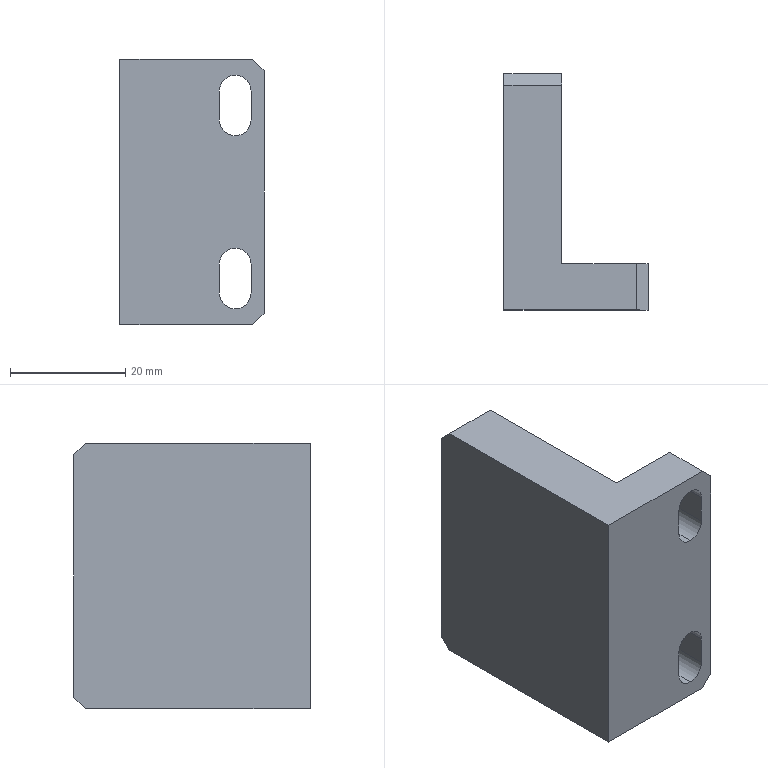Part | SolidWorks | features Chamfer 1, Extrusion 1, HoleWzd 1, ICE 1 | 1 solid | 30 faces | box 25 x 41 x 46 mm | volume 23309 mm3 | plane 16 | cylinder 10 | cone 4 | commonest cylinder face diameters 5.5 x6 3.3 x4
STEP:
#1=CARTESIAN_POINT('',(5.,30.9,-19.15));
#2=VERTEX_POINT('',#1);
#3=CARTESIAN_POINT('',(5.,30.9,-15.85));
#4=VERTEX_POINT('',#3);
#5=CARTESIAN_POINT('',(5.,30.9,-17.5));
#6=DIRECTION('',(0.,1.,0.));
#7=DIRECTION('',(0.,0.,1.));
#8=AXIS2_PLACEMENT_3D('',#5,#6,#7);
#9=CIRCLE('',#8,1.65);
#10=EDGE_CURVE('',#2,#4,#9,.T.);
#11=ORIENTED_EDGE('',*,*,#10,.F.);
#12=CARTESIAN_POINT('',(5.,41.,-19.15));
#13=VERTEX_POINT('',#12);
#14=CARTESIAN_POINT('',(5.,41.,-19.15));
#15=DIRECTION('',(0.,1.,0.));
#16=VECTOR('',#15,1000.);
#17=LINE('',#14,#16);
#18=EDGE_CURVE('',#2,#13,#17,.T.);
#19=ORIENTED_EDGE('',*,*,#18,.T.);
#20=CARTESIAN_POINT('',(5.,41.,-15.85));
#21=VERTEX_POINT('',#20);
#22=CARTESIAN_POINT('',(5.,41.,-17.5));
#23=DIRECTION('',(0.,1.,0.));
#24=DIRECTION('',(0.,0.,1.));
#25=AXIS2_PLACEMENT_3D('',#22,#23,#24);
#26=CIRCLE('',#25,1.65);
#27=EDGE_CURVE('',#13,#21,#26,.T.);
#28=ORIENTED_EDGE('',*,*,#27,.T.);
#29=CARTESIAN_POINT('',(5.,41.,-15.85));
#30=DIRECTION('',(0.,1.,0.));
#31=VECTOR('',#30,1000.);
#32=LINE('',#29,#31);
#33=EDGE_CURVE('',#4,#21,#32,.T.);
#34=ORIENTED_EDGE('',*,*,#33,.F.);
#35=EDGE_LOOP('',(#11,#19,#28,#34));
#36=FACE_OUTER_BOUND('',#35,.T.);
#37=CARTESIAN_POINT('',(5.,41.,-17.5));
#38=DIRECTION('',(0.,1.,0.));
#39=DIRECTION('',(0.,0.,1.));
#40=AXIS2_PLACEMENT_3D('',#37,#38,#39);
#41=CYLINDRICAL_SURFACE('',#40,1.65);
#42=ADVANCED_FACE('',(#36),#41,.F.);
#43=CARTESIAN_POINT('',(5.,29.909,-17.5));
#44=VERTEX_POINT('',#43);
#45=CARTESIAN_POINT('',(5.,30.9,-15.85));
#46=DIRECTION('',(0.,0.515,0.8572));
#47=VECTOR('',#46,1000.);
#48=LINE('',#45,#47);
#49=EDGE_CURVE('',#44,#4,#48,.T.);
#50=ORIENTED_EDGE('',*,*,#49,.F.);
#51=CARTESIAN_POINT('',(5.,30.9,-19.15));
#52=DIRECTION('',(0.,0.515,-0.8572));
#53=VECTOR('',#52,1000.);
#54=LINE('',#51,#53);
#55=EDGE_CURVE('',#44,#2,#54,.T.);
#56=ORIENTED_EDGE('',*,*,#55,.T.);
#57=ORIENTED_EDGE('',*,*,#10,.T.);
#58=EDGE_LOOP('',(#50,#56,#57));
#59=FACE_OUTER_BOUND('',#58,.T.);
#60=CARTESIAN_POINT('',(5.,30.9,-17.5));
#61=DIRECTION('',(0.,1.,0.));
#62=DIRECTION('',(0.,0.,1.));
#63=AXIS2_PLACEMENT_3D('',#60,#61,#62);
#64=CONICAL_SURFACE('',#63,1.65,1.03);
#65=ADVANCED_FACE('',(#59),#64,.F.);
#66=CARTESIAN_POINT('',(5.,30.9,15.85));
#67=VERTEX_POINT('',#66);
#68=CARTESIAN_POINT('',(5.,30.9,19.15));
#69=VERTEX_POINT('',#68);
#70=CARTESIAN_POINT('',(5.,30.9,17.5));
#71=DIRECTION('',(0.,1.,0.));
#72=DIRECTION('',(0.,0.,1.));
#73=AXIS2_PLACEMENT_3D('',#70,#71,#72);
#74=CIRCLE('',#73,1.65);
#75=EDGE_CURVE('',#67,#69,#74,.T.);
#76=ORIENTED_EDGE('',*,*,#75,.F.);
#77=CARTESIAN_POINT('',(5.,41.,15.85));
#78=VERTEX_POINT('',#77);
#79=CARTESIAN_POINT('',(5.,41.,15.85));
#80=DIRECTION('',(0.,1.,0.));
#81=VECTOR('',#80,1000.);
#82=LINE('',#79,#81);
#83=EDGE_CURVE('',#67,#78,#82,.T.);
#84=ORIENTED_EDGE('',*,*,#83,.T.);
#85=CARTESIAN_POINT('',(5.,41.,19.15));
#86=VERTEX_POINT('',#85);
#87=CARTESIAN_POINT('',(5.,41.,17.5));
#88=DIRECTION('',(0.,1.,0.));
#89=DIRECTION('',(0.,0.,1.));
#90=AXIS2_PLACEMENT_3D('',#87,#88,#89);
#91=CIRCLE('',#90,1.65);
#92=EDGE_CURVE('',#78,#86,#91,.T.);
#93=ORIENTED_EDGE('',*,*,#92,.T.);
#94=CARTESIAN_POINT('',(5.,41.,19.15));
#95=DIRECTION('',(0.,1.,0.));
#96=VECTOR('',#95,1000.);
#97=LINE('',#94,#96);
#98=EDGE_CURVE('',#69,#86,#97,.T.);
#99=ORIENTED_EDGE('',*,*,#98,.F.);
#100=EDGE_LOOP('',(#76,#84,#93,#99));
#101=FACE_OUTER_BOUND('',#100,.T.);
#102=CARTESIAN_POINT('',(5.,41.,17.5));
#103=DIRECTION('',(0.,1.,0.));
#104=DIRECTION('',(0.,0.,1.));
#105=AXIS2_PLACEMENT_3D('',#102,#103,#104);
#106=CYLINDRICAL_SURFACE('',#105,1.65);
#107=ADVANCED_FACE('',(#101),#106,.F.);
#108=CARTESIAN_POINT('',(5.,29.909,17.5));
#109=VERTEX_POINT('',#108);
#110=CARTESIAN_POINT('',(5.,30.9,19.15));
#111=DIRECTION('',(0.,0.515,0.8572));
#112=VECTOR('',#111,1000.);
#113=LINE('',#110,#112);
#114=EDGE_CURVE('',#109,#69,#113,.T.);
#115=ORIENTED_EDGE('',*,*,#114,.F.);
#116=CARTESIAN_POINT('',(5.,30.9,15.85));
#117=DIRECTION('',(0.,0.515,-0.8572));
#118=VECTOR('',#117,1000.);
#119=LINE('',#116,#118);
#120=EDGE_CURVE('',#109,#67,#119,.T.);
#121=ORIENTED_EDGE('',*,*,#120,.T.);
#122=ORIENTED_EDGE('',*,*,#75,.T.);
#123=EDGE_LOOP('',(#115,#121,#122));
#124=FACE_OUTER_BOUND('',#123,.T.);
#125=CARTESIAN_POINT('',(5.,30.9,17.5));
#126=DIRECTION('',(0.,1.,0.));
#127=DIRECTION('',(0.,0.,1.));
#128=AXIS2_PLACEMENT_3D('',#125,#126,#127);
#129=CONICAL_SURFACE('',#128,1.65,1.03);
#130=ADVANCED_FACE('',(#124),#129,.F.);
#131=CARTESIAN_POINT('',(22.75,8.,12.5));
#132=VERTEX_POINT('',#131);
#133=CARTESIAN_POINT('',(20.,8.,9.75));
#134=VERTEX_POINT('',#133);
#135=CARTESIAN_POINT('',(20.,8.,12.5));
#136=DIRECTION('',(0.,1.,0.));
#137=DIRECTION('',(1.,0.,0.));
#138=AXIS2_PLACEMENT_3D('',#135,#136,#137);
#139=CIRCLE('',#138,2.75);
#140=EDGE_CURVE('',#132,#134,#139,.T.);
#141=ORIENTED_EDGE('',*,*,#140,.T.);
#142=CARTESIAN_POINT('',(20.,0.,9.75));
#143=VERTEX_POINT('',#142);
#144=CARTESIAN_POINT('',(20.,41.,9.75));
#145=DIRECTION('',(0.,-1.,0.));
#146=VECTOR('',#145,1000.);
#147=LINE('',#144,#146);
#148=EDGE_CURVE('',#134,#143,#147,.T.);
#149=ORIENTED_EDGE('',*,*,#148,.T.);
#150=CARTESIAN_POINT('',(22.75,0.,12.5));
#151=VERTEX_POINT('',#150);
#152=CARTESIAN_POINT('',(20.,0.,12.5));
#153=DIRECTION('',(0.,1.,0.));
#154=DIRECTION('',(0.,0.,1.));
#155=AXIS2_PLACEMENT_3D('',#152,#153,#154);
#156=CIRCLE('',#155,2.75);
#157=EDGE_CURVE('',#151,#143,#156,.T.);
#158=ORIENTED_EDGE('',*,*,#157,.F.);
#159=CARTESIAN_POINT('',(22.75,41.,12.5));
#160=DIRECTION('',(0.,-1.,0.));
#161=VECTOR('',#160,1000.);
#162=LINE('',#159,#161);
#163=EDGE_CURVE('',#132,#151,#162,.T.);
#164=ORIENTED_EDGE('',*,*,#163,.F.);
#165=EDGE_LOOP('',(#141,#149,#158,#164));
#166=FACE_OUTER_BOUND('',#165,.T.);
#167=CARTESIAN_POINT('',(20.,41.,12.5));
#168=DIRECTION('',(0.,-1.,0.));
#169=DIRECTION('',(0.,0.,-1.));
#170=AXIS2_PLACEMENT_3D('',#167,#168,#169);
#171=CYLINDRICAL_SURFACE('',#170,2.75);
#172=ADVANCED_FACE('',(#166),#171,.F.);
#173=CARTESIAN_POINT('',(22.75,8.,-17.5));
#174=VERTEX_POINT('',#173);
#175=CARTESIAN_POINT('',(20.,8.,-20.25));
#176=VERTEX_POINT('',#175);
#177=CARTESIAN_POINT('',(20.,8.,-17.5));
#178=DIRECTION('',(0.,1.,0.));
#179=DIRECTION('',(1.,0.,0.));
#180=AXIS2_PLACEMENT_3D('',#177,#178,#179);
#181=CIRCLE('',#180,2.75);
#182=EDGE_CURVE('',#174,#176,#181,.T.);
#183=ORIENTED_EDGE('',*,*,#182,.T.);
#184=CARTESIAN_POINT('',(20.,0.,-20.25));
#185=VERTEX_POINT('',#184);
#186=CARTESIAN_POINT('',(20.,41.,-20.25));
#187=DIRECTION('',(0.,-1.,0.));
#188=VECTOR('',#187,1000.);
#189=LINE('',#186,#188);
#190=EDGE_CURVE('',#176,#185,#189,.T.);
#191=ORIENTED_EDGE('',*,*,#190,.T.);
#192=CARTESIAN_POINT('',(22.75,0.,-17.5));
#193=VERTEX_POINT('',#192);
#194=CARTESIAN_POINT('',(20.,0.,-17.5));
#195=DIRECTION('',(0.,1.,0.));
#196=DIRECTION('',(0.,0.,1.));
#197=AXIS2_PLACEMENT_3D('',#194,#195,#196);
#198=CIRCLE('',#197,2.75);
#199=EDGE_CURVE('',#193,#185,#198,.T.);
#200=ORIENTED_EDGE('',*,*,#199,.F.);
#201=CARTESIAN_POINT('',(22.75,41.,-17.5));
#202=DIRECTION('',(0.,-1.,0.));
#203=VECTOR('',#202,1000.);
#204=LINE('',#201,#203);
#205=EDGE_CURVE('',#174,#193,#204,.T.);
#206=ORIENTED_EDGE('',*,*,#205,.F.);
#207=EDGE_LOOP('',(#183,#191,#200,#206));
#208=FACE_OUTER_BOUND('',#207,.T.);
#209=CARTESIAN_POINT('',(20.,41.,-17.5));
#210=DIRECTION('',(0.,-1.,0.));
#211=DIRECTION('',(0.,0.,-1.));
#212=AXIS2_PLACEMENT_3D('',#209,#210,#211);
#213=CYLINDRICAL_SURFACE('',#212,2.75);
#214=ADVANCED_FACE('',(#208),#213,.F.);
#215=ORIENTED_EDGE('',*,*,#199,.T.);
#216=CARTESIAN_POINT('',(17.25,0.,-17.5));
#217=VERTEX_POINT('',#216);
#218=CARTESIAN_POINT('',(20.,0.,-17.5));
#219=DIRECTION('',(0.,1.,0.));
#220=DIRECTION('',(0.,0.,1.));
#221=AXIS2_PLACEMENT_3D('',#218,#219,#220);
#222=CIRCLE('',#221,2.75);
#223=EDGE_CURVE('',#185,#217,#222,.T.);
#224=ORIENTED_EDGE('',*,*,#223,.T.);
#225=CARTESIAN_POINT('',(17.25,0.,-12.5));
#226=VERTEX_POINT('',#225);
#227=CARTESIAN_POINT('',(17.25,0.,-17.5));
#228=DIRECTION('',(0.,0.,1.));
#229=VECTOR('',#228,1000.);
#230=LINE('',#227,#229);
#231=EDGE_CURVE('',#217,#226,#230,.T.);
#232=ORIENTED_EDGE('',*,*,#231,.T.);
#233=CARTESIAN_POINT('',(22.75,0.,-12.5));
#234=VERTEX_POINT('',#233);
#235=CARTESIAN_POINT('',(20.,0.,-12.5));
#236=DIRECTION('',(0.,1.,0.));
#237=DIRECTION('',(0.,0.,1.));
#238=AXIS2_PLACEMENT_3D('',#235,#236,#237);
#239=CIRCLE('',#238,2.75);
#240=EDGE_CURVE('',#226,#234,#239,.T.);
#241=ORIENTED_EDGE('',*,*,#240,.T.);
#242=CARTESIAN_POINT('',(22.75,0.,-17.5));
#243=DIRECTION('',(0.,0.,-1.));
#244=VECTOR('',#243,1000.);
#245=LINE('',#242,#244);
#246=EDGE_CURVE('',#234,#193,#245,.T.);
#247=ORIENTED_EDGE('',*,*,#246,.T.);
#248=EDGE_LOOP('',(#215,#224,#232,#241,#247));
#249=FACE_BOUND('',#248,.T.);
#250=CARTESIAN_POINT('',(25.,0.,21.));
#251=VERTEX_POINT('',#250);
#252=CARTESIAN_POINT('',(25.,0.,-21.));
#253=VERTEX_POINT('',#252);
#254=CARTESIAN_POINT('',(25.,0.,23.));
#255=DIRECTION('',(0.,0.,-1.));
#256=VECTOR('',#255,1000.);
#257=LINE('',#254,#256);
#258=EDGE_CURVE('',#251,#253,#257,.T.);
#259=ORIENTED_EDGE('',*,*,#258,.F.);
#260=CARTESIAN_POINT('',(23.,0.,23.));
#261=VERTEX_POINT('',#260);
#262=CARTESIAN_POINT('',(23.,0.,23.));
#263=DIRECTION('',(-0.7071,0.,0.7071));
#264=VECTOR('',#263,1000.);
#265=LINE('',#262,#264);
#266=EDGE_CURVE('',#251,#261,#265,.T.);
#267=ORIENTED_EDGE('',*,*,#266,.T.);
#268=CARTESIAN_POINT('',(0.,0.,23.));
#269=VERTEX_POINT('',#268);
#270=CARTESIAN_POINT('',(0.,0.,23.));
#271=DIRECTION('',(1.,0.,0.));
#272=VECTOR('',#271,1000.);
#273=LINE('',#270,#272);
#274=EDGE_CURVE('',#269,#261,#273,.T.);
#275=ORIENTED_EDGE('',*,*,#274,.F.);
#276=CARTESIAN_POINT('',(0.,0.,-23.));
#277=VERTEX_POINT('',#276);
#278=CARTESIAN_POINT('',(0.,0.,23.));
#279=DIRECTION('',(0.,0.,-1.));
#280=VECTOR('',#279,1000.);
#281=LINE('',#278,#280);
#282=EDGE_CURVE('',#269,#277,#281,.T.);
#283=ORIENTED_EDGE('',*,*,#282,.T.);
#284=CARTESIAN_POINT('',(23.,0.,-23.));
#285=VERTEX_POINT('',#284);
#286=CARTESIAN_POINT('',(0.,0.,-23.));
#287=DIRECTION('',(1.,0.,0.));
#288=VECTOR('',#287,1000.);
#289=LINE('',#286,#288);
#290=EDGE_CURVE('',#277,#285,#289,.T.);
#291=ORIENTED_EDGE('',*,*,#290,.T.);
#292=CARTESIAN_POINT('',(25.,0.,-21.));
#293=DIRECTION('',(0.7071,0.,0.7071));
#294=VECTOR('',#293,1000.);
#295=LINE('',#292,#294);
#296=EDGE_CURVE('',#285,#253,#295,.T.);
#297=ORIENTED_EDGE('',*,*,#296,.T.);
#298=EDGE_LOOP('',(#259,#267,#275,#283,#291,#297));
#299=FACE_OUTER_BOUND('',#298,.T.);
#300=ORIENTED_EDGE('',*,*,#157,.T.);
#301=CARTESIAN_POINT('',(17.25,0.,12.5));
#302=VERTEX_POINT('',#301);
#303=CARTESIAN_POINT('',(20.,0.,12.5));
#304=DIRECTION('',(0.,1.,0.));
#305=DIRECTION('',(0.,0.,1.));
#306=AXIS2_PLACEMENT_3D('',#303,#304,#305);
#307=CIRCLE('',#306,2.75);
#308=EDGE_CURVE('',#143,#302,#307,.T.);
#309=ORIENTED_EDGE('',*,*,#308,.T.);
#310=CARTESIAN_POINT('',(17.25,0.,17.5));
#311=VERTEX_POINT('',#310);
#312=CARTESIAN_POINT('',(17.25,0.,12.5));
#313=DIRECTION('',(0.,0.,1.));
#314=VECTOR('',#313,1000.);
#315=LINE('',#312,#314);
#316=EDGE_CURVE('',#302,#311,#315,.T.);
#317=ORIENTED_EDGE('',*,*,#316,.T.);
#318=CARTESIAN_POINT('',(22.75,0.,17.5));
#319=VERTEX_POINT('',#318);
#320=CARTESIAN_POINT('',(20.,0.,17.5));
#321=DIRECTION('',(0.,1.,0.));
#322=DIRECTION('',(0.,0.,1.));
#323=AXIS2_PLACEMENT_3D('',#320,#321,#322);
#324=CIRCLE('',#323,2.75);
#325=EDGE_CURVE('',#311,#319,#324,.T.);
#326=ORIENTED_EDGE('',*,*,#325,.T.);
#327=CARTESIAN_POINT('',(22.75,0.,12.5));
#328=DIRECTION('',(0.,0.,-1.));
#329=VECTOR('',#328,1000.);
#330=LINE('',#327,#329);
#331=EDGE_CURVE('',#319,#151,#330,.T.);
#332=ORIENTED_EDGE('',*,*,#331,.T.);
#333=EDGE_LOOP('',(#300,#309,#317,#326,#332));
#334=FACE_BOUND('',#333,.T.);
#335=CARTESIAN_POINT('',(0.,0.,23.));
#336=DIRECTION('',(0.,1.,0.));
#337=DIRECTION('',(0.,0.,1.));
#338=AXIS2_PLACEMENT_3D('',#335,#336,#337);
#339=PLANE('',#338);
#340=ADVANCED_FACE('',(#249,#299,#334),#339,.F.);
#341=ORIENTED_EDGE('',*,*,#182,.F.);
#342=CARTESIAN_POINT('',(22.75,8.,-12.5));
#343=VERTEX_POINT('',#342);
#344=CARTESIAN_POINT('',(22.75,8.,23.));
#345=DIRECTION('',(0.,0.,-1.));
#346=VECTOR('',#345,1000.);
#347=LINE('',#344,#346);
#348=EDGE_CURVE('',#343,#174,#347,.T.);
#349=ORIENTED_EDGE('',*,*,#348,.F.);
#350=CARTESIAN_POINT('',(17.25,8.,-12.5));
#351=VERTEX_POINT('',#350);
#352=CARTESIAN_POINT('',(20.,8.,-12.5));
#353=DIRECTION('',(0.,1.,0.));
#354=DIRECTION('',(1.,0.,0.));
#355=AXIS2_PLACEMENT_3D('',#352,#353,#354);
#356=CIRCLE('',#355,2.75);
#357=EDGE_CURVE('',#351,#343,#356,.T.);
#358=ORIENTED_EDGE('',*,*,#357,.F.);
#359=CARTESIAN_POINT('',(17.25,8.,-17.5));
#360=VERTEX_POINT('',#359);
#361=CARTESIAN_POINT('',(17.25,8.,23.));
#362=DIRECTION('',(0.,0.,1.));
#363=VECTOR('',#362,1000.);
#364=LINE('',#361,#363);
#365=EDGE_CURVE('',#360,#351,#364,.T.);
#366=ORIENTED_EDGE('',*,*,#365,.F.);
#367=CARTESIAN_POINT('',(20.,8.,-17.5));
#368=DIRECTION('',(0.,1.,0.));
#369=DIRECTION('',(1.,0.,0.));
#370=AXIS2_PLACEMENT_3D('',#367,#368,#369);
#371=CIRCLE('',#370,2.75);
#372=EDGE_CURVE('',#176,#360,#371,.T.);
#373=ORIENTED_EDGE('',*,*,#372,.F.);
#374=EDGE_LOOP('',(#341,#349,#358,#366,#373));
#375=FACE_BOUND('',#374,.T.);
#376=CARTESIAN_POINT('',(23.,8.,23.));
#377=VERTEX_POINT('',#376);
#378=CARTESIAN_POINT('',(10.,8.,23.));
#379=VERTEX_POINT('',#378);
#380=CARTESIAN_POINT('',(25.,8.,23.));
#381=DIRECTION('',(-1.,0.,0.));
#382=VECTOR('',#381,1000.);
#383=LINE('',#380,#382);
#384=EDGE_CURVE('',#377,#379,#383,.T.);
#385=ORIENTED_EDGE('',*,*,#384,.F.);
#386=CARTESIAN_POINT('',(25.,8.,21.));
#387=VERTEX_POINT('',#386);
#388=CARTESIAN_POINT('',(23.,8.,23.));
#389=DIRECTION('',(0.7071,0.,-0.7071));
#390=VECTOR('',#389,1000.);
#391=LINE('',#388,#390);
#392=EDGE_CURVE('',#377,#387,#391,.T.);
#393=ORIENTED_EDGE('',*,*,#392,.T.);
#394=CARTESIAN_POINT('',(25.,8.,-21.));
#395=VERTEX_POINT('',#394);
#396=CARTESIAN_POINT('',(25.,8.,23.));
#397=DIRECTION('',(0.,0.,-1.));
#398=VECTOR('',#397,1000.);
#399=LINE('',#396,#398);
#400=EDGE_CURVE('',#387,#395,#399,.T.);
#401=ORIENTED_EDGE('',*,*,#400,.T.);
#402=CARTESIAN_POINT('',(23.,8.,-23.));
#403=VERTEX_POINT('',#402);
#404=CARTESIAN_POINT('',(25.,8.,-21.));
#405=DIRECTION('',(-0.7071,0.,-0.7071));
#406=VECTOR('',#405,1000.);
#407=LINE('',#404,#406);
#408=EDGE_CURVE('',#395,#403,#407,.T.);
#409=ORIENTED_EDGE('',*,*,#408,.T.);
#410=CARTESIAN_POINT('',(10.,8.,-23.));
#411=VERTEX_POINT('',#410);
#412=CARTESIAN_POINT('',(25.,8.,-23.));
#413=DIRECTION('',(-1.,0.,0.));
#414=VECTOR('',#413,1000.);
#415=LINE('',#412,#414);
#416=EDGE_CURVE('',#403,#411,#415,.T.);
#417=ORIENTED_EDGE('',*,*,#416,.T.);
#418=CARTESIAN_POINT('',(10.,8.,23.));
#419=DIRECTION('',(0.,0.,-1.));
#420=VECTOR('',#419,1000.);
#421=LINE('',#418,#420);
#422=EDGE_CURVE('',#379,#411,#421,.T.);
#423=ORIENTED_EDGE('',*,*,#422,.F.);
#424=EDGE_LOOP('',(#385,#393,#401,#409,#417,#423));
#425=FACE_OUTER_BOUND('',#424,.T.);
#426=ORIENTED_EDGE('',*,*,#140,.F.);
#427=CARTESIAN_POINT('',(22.75,8.,17.5));
#428=VERTEX_POINT('',#427);
#429=CARTESIAN_POINT('',(22.75,8.,23.));
#430=DIRECTION('',(0.,0.,-1.));
#431=VECTOR('',#430,1000.);
#432=LINE('',#429,#431);
#433=EDGE_CURVE('',#428,#132,#432,.T.);
#434=ORIENTED_EDGE('',*,*,#433,.F.);
#435=CARTESIAN_POINT('',(17.25,8.,17.5));
#436=VERTEX_POINT('',#435);
#437=CARTESIAN_POINT('',(20.,8.,17.5));
#438=DIRECTION('',(0.,1.,0.));
#439=DIRECTION('',(1.,0.,0.));
#440=AXIS2_PLACEMENT_3D('',#437,#438,#439);
#441=CIRCLE('',#440,2.75);
#442=EDGE_CURVE('',#436,#428,#441,.T.);
#443=ORIENTED_EDGE('',*,*,#442,.F.);
#444=CARTESIAN_POINT('',(17.25,8.,12.5));
#445=VERTEX_POINT('',#444);
#446=CARTESIAN_POINT('',(17.25,8.,23.));
#447=DIRECTION('',(0.,0.,1.));
#448=VECTOR('',#447,1000.);
#449=LINE('',#446,#448);
#450=EDGE_CURVE('',#445,#436,#449,.T.);
#451=ORIENTED_EDGE('',*,*,#450,.F.);
#452=CARTESIAN_POINT('',(20.,8.,12.5));
#453=DIRECTION('',(0.,1.,0.));
#454=DIRECTION('',(1.,0.,0.));
#455=AXIS2_PLACEMENT_3D('',#452,#453,#454);
#456=CIRCLE('',#455,2.75);
#457=EDGE_CURVE('',#134,#445,#456,.T.);
#458=ORIENTED_EDGE('',*,*,#457,.F.);
#459=EDGE_LOOP('',(#426,#434,#443,#451,#458));
#460=FACE_BOUND('',#459,.T.);
#461=CARTESIAN_POINT('',(25.,8.,23.));
#462=DIRECTION('',(0.,-1.,0.));
#463=DIRECTION('',(1.,0.,0.));
#464=AXIS2_PLACEMENT_3D('',#461,#462,#463);
#465=PLANE('',#464);
#466=ADVANCED_FACE('',(#375,#425,#460),#465,.F.);
#467=CARTESIAN_POINT('',(0.,39.,23.));
#468=VERTEX_POINT('',#467);
#469=CARTESIAN_POINT('',(0.,0.,23.));
#470=DIRECTION('',(0.,-1.,0.));
#471=VECTOR('',#470,1000.);
#472=LINE('',#469,#471);
#473=EDGE_CURVE('',#468,#269,#472,.T.);
#474=ORIENTED_EDGE('',*,*,#473,.F.);
#475=CARTESIAN_POINT('',(0.,41.,21.));
#476=VERTEX_POINT('',#475);
#477=CARTESIAN_POINT('',(0.,39.,23.));
#478=DIRECTION('',(0.,0.7071,-0.7071));
#479=VECTOR('',#478,1000.);
#480=LINE('',#477,#479);
#481=EDGE_CURVE('',#468,#476,#480,.T.);
#482=ORIENTED_EDGE('',*,*,#481,.T.);
#483=CARTESIAN_POINT('',(0.,41.,-21.));
#484=VERTEX_POINT('',#483);
#485=CARTESIAN_POINT('',(0.,41.,23.));
#486=DIRECTION('',(0.,0.,-1.));
#487=VECTOR('',#486,1000.);
#488=LINE('',#485,#487);
#489=EDGE_CURVE('',#476,#484,#488,.T.);
#490=ORIENTED_EDGE('',*,*,#489,.T.);
#491=CARTESIAN_POINT('',(0.,39.,-23.));
#492=VERTEX_POINT('',#491);
#493=CARTESIAN_POINT('',(0.,41.,-21.));
#494=DIRECTION('',(0.,-0.7071,-0.7071));
#495=VECTOR('',#494,1000.);
#496=LINE('',#493,#495);
#497=EDGE_CURVE('',#484,#492,#496,.T.);
#498=ORIENTED_EDGE('',*,*,#497,.T.);
#499=CARTESIAN_POINT('',(0.,0.,-23.));
#500=DIRECTION('',(0.,-1.,0.));
#501=VECTOR('',#500,1000.);
#502=LINE('',#499,#501);
#503=EDGE_CURVE('',#492,#277,#502,.T.);
#504=ORIENTED_EDGE('',*,*,#503,.T.);
#505=ORIENTED_EDGE('',*,*,#282,.F.);
#506=EDGE_LOOP('',(#474,#482,#490,#498,#504,#505));
#507=FACE_OUTER_BOUND('',#506,.T.);
#508=CARTESIAN_POINT('',(0.,0.,23.));
#509=DIRECTION('',(1.,0.,0.));
#510=DIRECTION('',(0.,0.,-1.));
#511=AXIS2_PLACEMENT_3D('',#508,#509,#510);
#512=PLANE('',#511);
#513=ADVANCED_FACE('',(#507),#512,.F.);
#514=ORIENTED_EDGE('',*,*,#400,.F.);
#515=CARTESIAN_POINT('',(25.,8.,21.));
#516=DIRECTION('',(0.,-1.,0.));
#517=VECTOR('',#516,1000.);
#518=LINE('',#515,#517);
#519=EDGE_CURVE('',#387,#251,#518,.T.);
#520=ORIENTED_EDGE('',*,*,#519,.T.);
#521=ORIENTED_EDGE('',*,*,#258,.T.);
#522=CARTESIAN_POINT('',(25.,8.,-21.));
#523=DIRECTION('',(0.,1.,0.));
#524=VECTOR('',#523,1000.);
#525=LINE('',#522,#524);
#526=EDGE_CURVE('',#253,#395,#525,.T.);
#527=ORIENTED_EDGE('',*,*,#526,.T.);
#528=EDGE_LOOP('',(#514,#520,#521,#527));
#529=FACE_OUTER_BOUND('',#528,.T.);
#530=CARTESIAN_POINT('',(25.,8.,23.));
#531=DIRECTION('',(-1.,0.,0.));
#532=DIRECTION('',(0.,0.,1.));
#533=AXIS2_PLACEMENT_3D('',#530,#531,#532);
#534=PLANE('',#533);
#535=ADVANCED_FACE('',(#529),#534,.F.);
#536=CARTESIAN_POINT('',(10.,41.,21.));
#537=VERTEX_POINT('',#536);
#538=CARTESIAN_POINT('',(10.,41.,-21.));
#539=VERTEX_POINT('',#538);
#540=CARTESIAN_POINT('',(10.,41.,23.));
#541=DIRECTION('',(0.,0.,-1.));
#542=VECTOR('',#541,1000.);
#543=LINE('',#540,#542);
#544=EDGE_CURVE('',#537,#539,#543,.T.);
#545=ORIENTED_EDGE('',*,*,#544,.F.);
#546=CARTESIAN_POINT('',(10.,39.,23.));
#547=VERTEX_POINT('',#546);
#548=CARTESIAN_POINT('',(10.,39.,23.));
#549=DIRECTION('',(0.,-0.7071,0.7071));
#550=VECTOR('',#549,1000.);
#551=LINE('',#548,#550);
#552=EDGE_CURVE('',#537,#547,#551,.T.);
#553=ORIENTED_EDGE('',*,*,#552,.T.);
#554=CARTESIAN_POINT('',(10.,41.,23.));
#555=DIRECTION('',(0.,1.,0.));
#556=VECTOR('',#555,1000.);
#557=LINE('',#554,#556);
#558=EDGE_CURVE('',#379,#547,#557,.T.);
#559=ORIENTED_EDGE('',*,*,#558,.F.);
#560=ORIENTED_EDGE('',*,*,#422,.T.);
#561=CARTESIAN_POINT('',(10.,39.,-23.));
#562=VERTEX_POINT('',#561);
#563=CARTESIAN_POINT('',(10.,41.,-23.));
#564=DIRECTION('',(0.,1.,0.));
#565=VECTOR('',#564,1000.);
#566=LINE('',#563,#565);
#567=EDGE_CURVE('',#411,#562,#566,.T.);
#568=ORIENTED_EDGE('',*,*,#567,.T.);
#569=CARTESIAN_POINT('',(10.,41.,-21.));
#570=DIRECTION('',(0.,0.7071,0.7071));
#571=VECTOR('',#570,1000.);
#572=LINE('',#569,#571);
#573=EDGE_CURVE('',#562,#539,#572,.T.);
#574=ORIENTED_EDGE('',*,*,#573,.T.);
#575=EDGE_LOOP('',(#545,#553,#559,#560,#568,#574));
#576=FACE_OUTER_BOUND('',#575,.T.);
#577=CARTESIAN_POINT('',(10.,41.,23.));
#578=DIRECTION('',(-1.,0.,0.));
#579=DIRECTION('',(0.,-1.,0.));
#580=AXIS2_PLACEMENT_3D('',#577,#578,#579);
#581=PLANE('',#580);
#582=ADVANCED_FACE('',(#576),#581,.F.);
#583=CARTESIAN_POINT('',(5.,41.,-17.5));
#584=DIRECTION('',(0.,1.,0.));
#585=DIRECTION('',(0.,0.,1.));
#586=AXIS2_PLACEMENT_3D('',#583,#584,#585);
#587=CIRCLE('',#586,1.65);
#588=EDGE_CURVE('',#21,#13,#587,.T.);
#589=ORIENTED_EDGE('',*,*,#588,.F.);
#590=ORIENTED_EDGE('',*,*,#27,.F.);
#591=EDGE_LOOP('',(#589,#590));
#592=FACE_BOUND('',#591,.T.);
#593=CARTESIAN_POINT('',(5.,41.,17.5));
#594=DIRECTION('',(0.,1.,0.));
#595=DIRECTION('',(0.,0.,1.));
#596=AXIS2_PLACEMENT_3D('',#593,#594,#595);
#597=CIRCLE('',#596,1.65);
#598=EDGE_CURVE('',#86,#78,#597,.T.);
#599=ORIENTED_EDGE('',*,*,#598,.F.);
#600=ORIENTED_EDGE('',*,*,#92,.F.);
#601=EDGE_LOOP('',(#599,#600));
#602=FACE_BOUND('',#601,.T.);
#603=ORIENTED_EDGE('',*,*,#489,.F.);
#604=CARTESIAN_POINT('',(0.,41.,21.));
#605=DIRECTION('',(1.,0.,0.));
#606=VECTOR('',#605,1000.);
#607=LINE('',#604,#606);
#608=EDGE_CURVE('',#476,#537,#607,.T.);
#609=ORIENTED_EDGE('',*,*,#608,.T.);
#610=ORIENTED_EDGE('',*,*,#544,.T.);
#611=CARTESIAN_POINT('',(0.,41.,-21.));
#612=DIRECTION('',(-1.,0.,0.));
#613=VECTOR('',#612,1000.);
#614=LINE('',#611,#613);
#615=EDGE_CURVE('',#539,#484,#614,.T.);
#616=ORIENTED_EDGE('',*,*,#615,.T.);
#617=EDGE_LOOP('',(#603,#609,#610,#616));
#618=FACE_OUTER_BOUND('',#617,.T.);
#619=CARTESIAN_POINT('',(0.,41.,23.));
#620=DIRECTION('',(0.,-1.,0.));
#621=DIRECTION('',(0.,0.,-1.));
#622=AXIS2_PLACEMENT_3D('',#619,#620,#621);
#623=PLANE('',#622);
#624=ADVANCED_FACE('',(#592,#602,#618),#623,.F.);
#625=ORIENTED_EDGE('',*,*,#558,.T.);
#626=CARTESIAN_POINT('',(0.,39.,23.));
#627=DIRECTION('',(-1.,0.,0.));
#628=VECTOR('',#627,1000.);
#629=LINE('',#626,#628);
#630=EDGE_CURVE('',#547,#468,#629,.T.);
#631=ORIENTED_EDGE('',*,*,#630,.T.);
#632=ORIENTED_EDGE('',*,*,#473,.T.);
#633=ORIENTED_EDGE('',*,*,#274,.T.);
#634=CARTESIAN_POINT('',(23.,0.,23.));
#635=DIRECTION('',(0.,1.,0.));
#636=VECTOR('',#635,1000.);
#637=LINE('',#634,#636);
#638=EDGE_CURVE('',#261,#377,#637,.T.);
#639=ORIENTED_EDGE('',*,*,#638,.T.);
#640=ORIENTED_EDGE('',*,*,#384,.T.);
#641=EDGE_LOOP('',(#625,#631,#632,#633,#639,#640));
#642=FACE_OUTER_BOUND('',#641,.T.);
#643=CARTESIAN_POINT('',(0.,0.,23.));
#644=DIRECTION('',(0.,0.,-1.));
#645=DIRECTION('',(-1.,0.,0.));
#646=AXIS2_PLACEMENT_3D('',#643,#644,#645);
#647=PLANE('',#646);
#648=ADVANCED_FACE('',(#642),#647,.F.);
#649=ORIENTED_EDGE('',*,*,#503,.F.);
#650=CARTESIAN_POINT('',(10.,39.,-23.));
#651=DIRECTION('',(1.,0.,0.));
#652=VECTOR('',#651,1000.);
#653=LINE('',#650,#652);
#654=EDGE_CURVE('',#492,#562,#653,.T.);
#655=ORIENTED_EDGE('',*,*,#654,.T.);
#656=ORIENTED_EDGE('',*,*,#567,.F.);
#657=ORIENTED_EDGE('',*,*,#416,.F.);
#658=CARTESIAN_POINT('',(23.,0.,-23.));
#659=DIRECTION('',(0.,-1.,0.));
#660=VECTOR('',#659,1000.);
#661=LINE('',#658,#660);
#662=EDGE_CURVE('',#403,#285,#661,.T.);
#663=ORIENTED_EDGE('',*,*,#662,.T.);
#664=ORIENTED_EDGE('',*,*,#290,.F.);
#665=EDGE_LOOP('',(#649,#655,#656,#657,#663,#664));
#666=FACE_OUTER_BOUND('',#665,.T.);
#667=CARTESIAN_POINT('',(0.,0.,-23.));
#668=DIRECTION('',(0.,0.,-1.));
#669=DIRECTION('',(-1.,0.,0.));
#670=AXIS2_PLACEMENT_3D('',#667,#668,#669);
#671=PLANE('',#670);
#672=ADVANCED_FACE('',(#666),#671,.T.);
#673=ORIENTED_EDGE('',*,*,#190,.F.);
#674=ORIENTED_EDGE('',*,*,#372,.T.);
#675=CARTESIAN_POINT('',(17.25,41.,-17.5));
#676=DIRECTION('',(0.,-1.,0.));
#677=VECTOR('',#676,1000.);
#678=LINE('',#675,#677);
#679=EDGE_CURVE('',#360,#217,#678,.T.);
#680=ORIENTED_EDGE('',*,*,#679,.T.);
#681=ORIENTED_EDGE('',*,*,#223,.F.);
#682=EDGE_LOOP('',(#673,#674,#680,#681));
#683=FACE_OUTER_BOUND('',#682,.T.);
#684=CARTESIAN_POINT('',(20.,41.,-17.5));
#685=DIRECTION('',(0.,-1.,0.));
#686=DIRECTION('',(0.,0.,-1.));
#687=AXIS2_PLACEMENT_3D('',#684,#685,#686);
#688=CYLINDRICAL_SURFACE('',#687,2.75);
#689=ADVANCED_FACE('',(#683),#688,.F.);
#690=ORIENTED_EDGE('',*,*,#365,.T.);
#691=CARTESIAN_POINT('',(17.25,41.,-12.5));
#692=DIRECTION('',(0.,-1.,0.));
#693=VECTOR('',#692,1000.);
#694=LINE('',#691,#693);
#695=EDGE_CURVE('',#351,#226,#694,.T.);
#696=ORIENTED_EDGE('',*,*,#695,.T.);
#697=ORIENTED_EDGE('',*,*,#231,.F.);
#698=ORIENTED_EDGE('',*,*,#679,.F.);
#699=EDGE_LOOP('',(#690,#696,#697,#698));
#700=FACE_OUTER_BOUND('',#699,.T.);
#701=CARTESIAN_POINT('',(17.25,41.,-17.5));
#702=DIRECTION('',(1.,0.,0.));
#703=DIRECTION('',(0.,0.,-1.));
#704=AXIS2_PLACEMENT_3D('',#701,#702,#703);
#705=PLANE('',#704);
#706=ADVANCED_FACE('',(#700),#705,.T.);
#707=ORIENTED_EDGE('',*,*,#357,.T.);
#708=CARTESIAN_POINT('',(22.75,41.,-12.5));
#709=DIRECTION('',(0.,-1.,0.));
#710=VECTOR('',#709,1000.);
#711=LINE('',#708,#710);
#712=EDGE_CURVE('',#343,#234,#711,.T.);
#713=ORIENTED_EDGE('',*,*,#712,.T.);
#714=ORIENTED_EDGE('',*,*,#240,.F.);
#715=ORIENTED_EDGE('',*,*,#695,.F.);
#716=EDGE_LOOP('',(#707,#713,#714,#715));
#717=FACE_OUTER_BOUND('',#716,.T.);
#718=CARTESIAN_POINT('',(20.,41.,-12.5));
#719=DIRECTION('',(0.,-1.,0.));
#720=DIRECTION('',(0.,0.,-1.));
#721=AXIS2_PLACEMENT_3D('',#718,#719,#720);
#722=CYLINDRICAL_SURFACE('',#721,2.75);
#723=ADVANCED_FACE('',(#717),#722,.F.);
#724=ORIENTED_EDGE('',*,*,#348,.T.);
#725=ORIENTED_EDGE('',*,*,#205,.T.);
#726=ORIENTED_EDGE('',*,*,#246,.F.);
#727=ORIENTED_EDGE('',*,*,#712,.F.);
#728=EDGE_LOOP('',(#724,#725,#726,#727));
#729=FACE_OUTER_BOUND('',#728,.T.);
#730=CARTESIAN_POINT('',(22.75,41.,-17.5));
#731=DIRECTION('',(-1.,0.,0.));
#732=DIRECTION('',(0.,0.,1.));
#733=AXIS2_PLACEMENT_3D('',#730,#731,#732);
#734=PLANE('',#733);
#735=ADVANCED_FACE('',(#729),#734,.T.);
#736=ORIENTED_EDGE('',*,*,#148,.F.);
#737=ORIENTED_EDGE('',*,*,#457,.T.);
#738=CARTESIAN_POINT('',(17.25,41.,12.5));
#739=DIRECTION('',(0.,-1.,0.));
#740=VECTOR('',#739,1000.);
#741=LINE('',#738,#740);
#742=EDGE_CURVE('',#445,#302,#741,.T.);
#743=ORIENTED_EDGE('',*,*,#742,.T.);
#744=ORIENTED_EDGE('',*,*,#308,.F.);
#745=EDGE_LOOP('',(#736,#737,#743,#744));
#746=FACE_OUTER_BOUND('',#745,.T.);
#747=CARTESIAN_POINT('',(20.,41.,12.5));
#748=DIRECTION('',(0.,-1.,0.));
#749=DIRECTION('',(0.,0.,-1.));
#750=AXIS2_PLACEMENT_3D('',#747,#748,#749);
#751=CYLINDRICAL_SURFACE('',#750,2.75);
#752=ADVANCED_FACE('',(#746),#751,.F.);
#753=ORIENTED_EDGE('',*,*,#450,.T.);
#754=CARTESIAN_POINT('',(17.25,41.,17.5));
#755=DIRECTION('',(0.,-1.,0.));
#756=VECTOR('',#755,1000.);
#757=LINE('',#754,#756);
#758=EDGE_CURVE('',#436,#311,#757,.T.);
#759=ORIENTED_EDGE('',*,*,#758,.T.);
#760=ORIENTED_EDGE('',*,*,#316,.F.);
#761=ORIENTED_EDGE('',*,*,#742,.F.);
#762=EDGE_LOOP('',(#753,#759,#760,#761));
#763=FACE_OUTER_BOUND('',#762,.T.);
#764=CARTESIAN_POINT('',(17.25,41.,12.5));
#765=DIRECTION('',(1.,0.,0.));
#766=DIRECTION('',(0.,0.,-1.));
#767=AXIS2_PLACEMENT_3D('',#764,#765,#766);
#768=PLANE('',#767);
#769=ADVANCED_FACE('',(#763),#768,.T.);
#770=ORIENTED_EDGE('',*,*,#442,.T.);
#771=CARTESIAN_POINT('',(22.75,41.,17.5));
#772=DIRECTION('',(0.,-1.,0.));
#773=VECTOR('',#772,1000.);
#774=LINE('',#771,#773);
#775=EDGE_CURVE('',#428,#319,#774,.T.);
#776=ORIENTED_EDGE('',*,*,#775,.T.);
#777=ORIENTED_EDGE('',*,*,#325,.F.);
#778=ORIENTED_EDGE('',*,*,#758,.F.);
#779=EDGE_LOOP('',(#770,#776,#777,#778));
#780=FACE_OUTER_BOUND('',#779,.T.);
#781=CARTESIAN_POINT('',(20.,41.,17.5));
#782=DIRECTION('',(0.,-1.,0.));
#783=DIRECTION('',(0.,0.,-1.));
#784=AXIS2_PLACEMENT_3D('',#781,#782,#783);
#785=CYLINDRICAL_SURFACE('',#784,2.75);
#786=ADVANCED_FACE('',(#780),#785,.F.);
#787=ORIENTED_EDGE('',*,*,#433,.T.);
#788=ORIENTED_EDGE('',*,*,#163,.T.);
#789=ORIENTED_EDGE('',*,*,#331,.F.);
#790=ORIENTED_EDGE('',*,*,#775,.F.);
#791=EDGE_LOOP('',(#787,#788,#789,#790));
#792=FACE_OUTER_BOUND('',#791,.T.);
#793=CARTESIAN_POINT('',(22.75,41.,12.5));
#794=DIRECTION('',(-1.,0.,0.));
#795=DIRECTION('',(0.,0.,1.));
#796=AXIS2_PLACEMENT_3D('',#793,#794,#795);
#797=PLANE('',#796);
#798=ADVANCED_FACE('',(#792),#797,.T.);
#799=ORIENTED_EDGE('',*,*,#120,.F.);
#800=ORIENTED_EDGE('',*,*,#114,.T.);
#801=CARTESIAN_POINT('',(5.,30.9,17.5));
#802=DIRECTION('',(0.,1.,0.));
#803=DIRECTION('',(0.,0.,1.));
#804=AXIS2_PLACEMENT_3D('',#801,#802,#803);
#805=CIRCLE('',#804,1.65);
#806=EDGE_CURVE('',#69,#67,#805,.T.);
#807=ORIENTED_EDGE('',*,*,#806,.T.);
#808=EDGE_LOOP('',(#799,#800,#807));
#809=FACE_OUTER_BOUND('',#808,.T.);
#810=CARTESIAN_POINT('',(5.,30.9,17.5));
#811=DIRECTION('',(0.,1.,0.));
#812=DIRECTION('',(0.,0.,1.));
#813=AXIS2_PLACEMENT_3D('',#810,#811,#812);
#814=CONICAL_SURFACE('',#813,1.65,1.03);
#815=ADVANCED_FACE('',(#809),#814,.F.);
#816=ORIENTED_EDGE('',*,*,#83,.F.);
#817=ORIENTED_EDGE('',*,*,#806,.F.);
#818=ORIENTED_EDGE('',*,*,#98,.T.);
#819=ORIENTED_EDGE('',*,*,#598,.T.);
#820=EDGE_LOOP('',(#816,#817,#818,#819));
#821=FACE_OUTER_BOUND('',#820,.T.);
#822=CARTESIAN_POINT('',(5.,41.,17.5));
#823=DIRECTION('',(0.,1.,0.));
#824=DIRECTION('',(0.,0.,1.));
#825=AXIS2_PLACEMENT_3D('',#822,#823,#824);
#826=CYLINDRICAL_SURFACE('',#825,1.65);
#827=ADVANCED_FACE('',(#821),#826,.F.);
#828=ORIENTED_EDGE('',*,*,#55,.F.);
#829=ORIENTED_EDGE('',*,*,#49,.T.);
#830=CARTESIAN_POINT('',(5.,30.9,-17.5));
#831=DIRECTION('',(0.,1.,0.));
#832=DIRECTION('',(0.,0.,1.));
#833=AXIS2_PLACEMENT_3D('',#830,#831,#832);
#834=CIRCLE('',#833,1.65);
#835=EDGE_CURVE('',#4,#2,#834,.T.);
#836=ORIENTED_EDGE('',*,*,#835,.T.);
#837=EDGE_LOOP('',(#828,#829,#836));
#838=FACE_OUTER_BOUND('',#837,.T.);
#839=CARTESIAN_POINT('',(5.,30.9,-17.5));
#840=DIRECTION('',(0.,1.,0.));
#841=DIRECTION('',(0.,0.,1.));
#842=AXIS2_PLACEMENT_3D('',#839,#840,#841);
#843=CONICAL_SURFACE('',#842,1.65,1.03);
#844=ADVANCED_FACE('',(#838),#843,.F.);
#845=ORIENTED_EDGE('',*,*,#18,.F.);
#846=ORIENTED_EDGE('',*,*,#835,.F.);
#847=ORIENTED_EDGE('',*,*,#33,.T.);
#848=ORIENTED_EDGE('',*,*,#588,.T.);
#849=EDGE_LOOP('',(#845,#846,#847,#848));
#850=FACE_OUTER_BOUND('',#849,.T.);
#851=CARTESIAN_POINT('',(5.,41.,-17.5));
#852=DIRECTION('',(0.,1.,0.));
#853=DIRECTION('',(0.,0.,1.));
#854=AXIS2_PLACEMENT_3D('',#851,#852,#853);
#855=CYLINDRICAL_SURFACE('',#854,1.65);
#856=ADVANCED_FACE('',(#850),#855,.F.);
#857=ORIENTED_EDGE('',*,*,#552,.F.);
#858=ORIENTED_EDGE('',*,*,#608,.F.);
#859=ORIENTED_EDGE('',*,*,#481,.F.);
#860=ORIENTED_EDGE('',*,*,#630,.F.);
#861=EDGE_LOOP('',(#857,#858,#859,#860));
#862=FACE_OUTER_BOUND('',#861,.T.);
#863=CARTESIAN_POINT('',(0.,39.,23.));
#864=DIRECTION('',(0.,-0.7071,-0.7071));
#865=DIRECTION('',(-1.,0.,0.));
#866=AXIS2_PLACEMENT_3D('',#863,#864,#865);
#867=PLANE('',#866);
#868=ADVANCED_FACE('',(#862),#867,.F.);
#869=ORIENTED_EDGE('',*,*,#573,.F.);
#870=ORIENTED_EDGE('',*,*,#654,.F.);
#871=ORIENTED_EDGE('',*,*,#497,.F.);
#872=ORIENTED_EDGE('',*,*,#615,.F.);
#873=EDGE_LOOP('',(#869,#870,#871,#872));
#874=FACE_OUTER_BOUND('',#873,.T.);
#875=CARTESIAN_POINT('',(0.,41.,-21.));
#876=DIRECTION('',(0.,0.7071,-0.7071));
#877=DIRECTION('',(1.,0.,0.));
#878=AXIS2_PLACEMENT_3D('',#875,#876,#877);
#879=PLANE('',#878);
#880=ADVANCED_FACE('',(#874),#879,.T.);
#881=ORIENTED_EDGE('',*,*,#266,.F.);
#882=ORIENTED_EDGE('',*,*,#519,.F.);
#883=ORIENTED_EDGE('',*,*,#392,.F.);
#884=ORIENTED_EDGE('',*,*,#638,.F.);
#885=EDGE_LOOP('',(#881,#882,#883,#884));
#886=FACE_OUTER_BOUND('',#885,.T.);
#887=CARTESIAN_POINT('',(23.,0.,23.));
#888=DIRECTION('',(-0.7071,0.,-0.7071));
#889=DIRECTION('',(0.,1.,0.));
#890=AXIS2_PLACEMENT_3D('',#887,#888,#889);
#891=PLANE('',#890);
#892=ADVANCED_FACE('',(#886),#891,.F.);
#893=ORIENTED_EDGE('',*,*,#296,.F.);
#894=ORIENTED_EDGE('',*,*,#662,.F.);
#895=ORIENTED_EDGE('',*,*,#408,.F.);
#896=ORIENTED_EDGE('',*,*,#526,.F.);
#897=EDGE_LOOP('',(#893,#894,#895,#896));
#898=FACE_OUTER_BOUND('',#897,.T.);
#899=CARTESIAN_POINT('',(25.,8.,-21.));
#900=DIRECTION('',(0.7071,0.,-0.7071));
#901=DIRECTION('',(0.,-1.,0.));
#902=AXIS2_PLACEMENT_3D('',#899,#900,#901);
#903=PLANE('',#902);
#904=ADVANCED_FACE('',(#898),#903,.T.);
#905=CLOSED_SHELL('',(#42,#65,#107,#130,#172,#214,#340,#466,#513,#535,#582,#624,#648,#672,#689,#706,#723,#735,#752,#769,#786,#798,#815,#827,#844,#856,#868,#880,#892,#904));
#906=MANIFOLD_SOLID_BREP('',#905);
#907=CARTESIAN_POINT('',(0.,0.,0.));
#908=DIRECTION('',(0.,0.,1.));
#909=DIRECTION('',(1.,0.,0.));
#910=AXIS2_PLACEMENT_3D('',#907,#908,#909);
#911=(LENGTH_UNIT()NAMED_UNIT(*)SI_UNIT(.MILLI.,.METRE.));
#912=UNCERTAINTY_MEASURE_WITH_UNIT(LENGTH_MEASURE(0.00001),#911,'','');
#913=(NAMED_UNIT(*)PLANE_ANGLE_UNIT()SI_UNIT($,.RADIAN.));
#914=(NAMED_UNIT(*)SI_UNIT($,.STERADIAN.)SOLID_ANGLE_UNIT());
#915=(GEOMETRIC_REPRESENTATION_CONTEXT(3)GLOBAL_UNCERTAINTY_ASSIGNED_CONTEXT((#912))GLOBAL_UNIT_ASSIGNED_CONTEXT((#911,#913,#914))REPRESENTATION_CONTEXT('',''));
#916=ADVANCED_BREP_SHAPE_REPRESENTATION('',(#906,#910),#915);